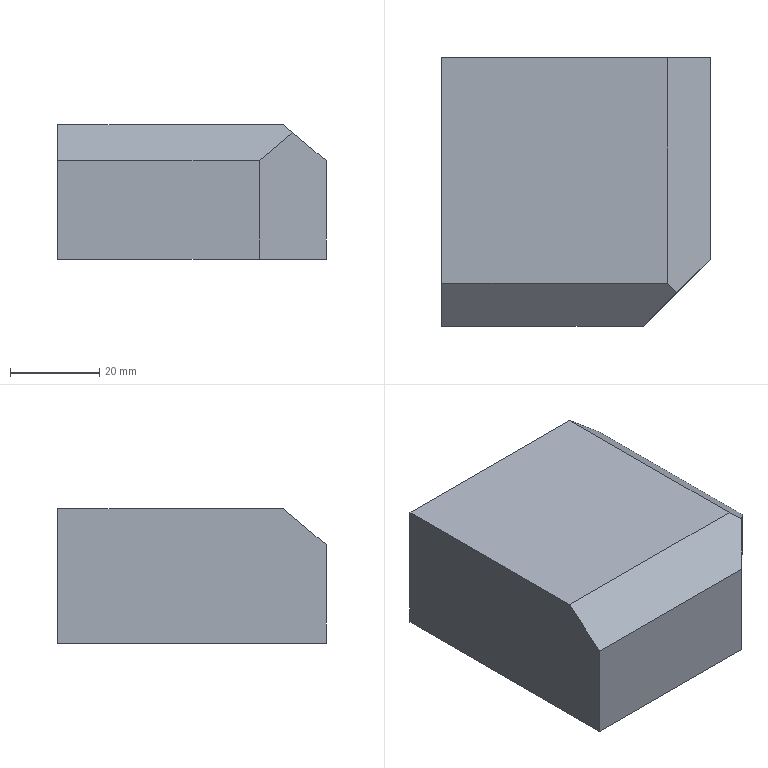Part | SolidWorks | features Chamfer 3, Extrusion 1 | 1 solid | 9 faces | box 60 x 60 x 30 mm | volume 100955 mm3 | plane 9
STEP:
#1=CARTESIAN_POINT('',(-30.,-30.,7.));
#2=VERTEX_POINT('',#1);
#3=CARTESIAN_POINT('',(-30.,-30.,-15.));
#4=VERTEX_POINT('',#3);
#5=CARTESIAN_POINT('',(-30.,-30.,15.));
#6=DIRECTION('',(0.,0.,-1.));
#7=VECTOR('',#6,1000.);
#8=LINE('',#5,#7);
#9=EDGE_CURVE('',#2,#4,#8,.T.);
#10=ORIENTED_EDGE('',*,*,#9,.F.);
#11=CARTESIAN_POINT('',(-30.,-20.466,15.));
#12=VERTEX_POINT('',#11);
#13=CARTESIAN_POINT('',(-30.,-20.466,15.));
#14=DIRECTION('',(0.,0.766,0.6428));
#15=VECTOR('',#14,1000.);
#16=LINE('',#13,#15);
#17=EDGE_CURVE('',#2,#12,#16,.T.);
#18=ORIENTED_EDGE('',*,*,#17,.T.);
#19=CARTESIAN_POINT('',(-30.,30.,15.));
#20=VERTEX_POINT('',#19);
#21=CARTESIAN_POINT('',(-30.,30.,15.));
#22=DIRECTION('',(0.,-1.,0.));
#23=VECTOR('',#22,1000.);
#24=LINE('',#21,#23);
#25=EDGE_CURVE('',#20,#12,#24,.T.);
#26=ORIENTED_EDGE('',*,*,#25,.F.);
#27=CARTESIAN_POINT('',(-30.,30.,-15.));
#28=VERTEX_POINT('',#27);
#29=CARTESIAN_POINT('',(-30.,30.,15.));
#30=DIRECTION('',(0.,0.,-1.));
#31=VECTOR('',#30,1000.);
#32=LINE('',#29,#31);
#33=EDGE_CURVE('',#20,#28,#32,.T.);
#34=ORIENTED_EDGE('',*,*,#33,.T.);
#35=CARTESIAN_POINT('',(-30.,30.,-15.));
#36=DIRECTION('',(0.,-1.,0.));
#37=VECTOR('',#36,1000.);
#38=LINE('',#35,#37);
#39=EDGE_CURVE('',#28,#4,#38,.T.);
#40=ORIENTED_EDGE('',*,*,#39,.T.);
#41=EDGE_LOOP('',(#10,#18,#26,#34,#40));
#42=FACE_OUTER_BOUND('',#41,.T.);
#43=CARTESIAN_POINT('',(-30.,30.,15.));
#44=DIRECTION('',(1.,0.,0.));
#45=DIRECTION('',(0.,1.,0.));
#46=AXIS2_PLACEMENT_3D('',#43,#44,#45);
#47=PLANE('',#46);
#48=ADVANCED_FACE('',(#42),#47,.F.);
#49=CARTESIAN_POINT('',(15.,-30.,-15.));
#50=VERTEX_POINT('',#49);
#51=CARTESIAN_POINT('',(15.,-30.,7.));
#52=VERTEX_POINT('',#51);
#53=CARTESIAN_POINT('',(15.,-30.,15.));
#54=DIRECTION('',(0.,0.,1.));
#55=VECTOR('',#54,1000.);
#56=LINE('',#53,#55);
#57=EDGE_CURVE('',#50,#52,#56,.T.);
#58=ORIENTED_EDGE('',*,*,#57,.T.);
#59=CARTESIAN_POINT('',(-30.,-30.,7.));
#60=DIRECTION('',(-1.,0.,0.));
#61=VECTOR('',#60,1000.);
#62=LINE('',#59,#61);
#63=EDGE_CURVE('',#52,#2,#62,.T.);
#64=ORIENTED_EDGE('',*,*,#63,.T.);
#65=ORIENTED_EDGE('',*,*,#9,.T.);
#66=CARTESIAN_POINT('',(-30.,-30.,-15.));
#67=DIRECTION('',(1.,0.,0.));
#68=VECTOR('',#67,1000.);
#69=LINE('',#66,#68);
#70=EDGE_CURVE('',#4,#50,#69,.T.);
#71=ORIENTED_EDGE('',*,*,#70,.T.);
#72=EDGE_LOOP('',(#58,#64,#65,#71));
#73=FACE_OUTER_BOUND('',#72,.T.);
#74=CARTESIAN_POINT('',(-30.,-30.,15.));
#75=DIRECTION('',(0.,1.,0.));
#76=DIRECTION('',(-1.,0.,0.));
#77=AXIS2_PLACEMENT_3D('',#74,#75,#76);
#78=PLANE('',#77);
#79=ADVANCED_FACE('',(#73),#78,.F.);
#80=CARTESIAN_POINT('',(30.,30.,7.));
#81=VERTEX_POINT('',#80);
#82=CARTESIAN_POINT('',(30.,30.,-15.));
#83=VERTEX_POINT('',#82);
#84=CARTESIAN_POINT('',(30.,30.,15.));
#85=DIRECTION('',(0.,0.,-1.));
#86=VECTOR('',#85,1000.);
#87=LINE('',#84,#86);
#88=EDGE_CURVE('',#81,#83,#87,.T.);
#89=ORIENTED_EDGE('',*,*,#88,.F.);
#90=CARTESIAN_POINT('',(30.,-15.,7.));
#91=VERTEX_POINT('',#90);
#92=CARTESIAN_POINT('',(30.,-15.,7.));
#93=DIRECTION('',(0.,-1.,0.));
#94=VECTOR('',#93,1000.);
#95=LINE('',#92,#94);
#96=EDGE_CURVE('',#81,#91,#95,.T.);
#97=ORIENTED_EDGE('',*,*,#96,.T.);
#98=CARTESIAN_POINT('',(30.,-15.,-15.));
#99=VERTEX_POINT('',#98);
#100=CARTESIAN_POINT('',(30.,-15.,15.));
#101=DIRECTION('',(0.,0.,-1.));
#102=VECTOR('',#101,1000.);
#103=LINE('',#100,#102);
#104=EDGE_CURVE('',#91,#99,#103,.T.);
#105=ORIENTED_EDGE('',*,*,#104,.T.);
#106=CARTESIAN_POINT('',(30.,30.,-15.));
#107=DIRECTION('',(0.,1.,0.));
#108=VECTOR('',#107,1000.);
#109=LINE('',#106,#108);
#110=EDGE_CURVE('',#99,#83,#109,.T.);
#111=ORIENTED_EDGE('',*,*,#110,.T.);
#112=EDGE_LOOP('',(#89,#97,#105,#111));
#113=FACE_OUTER_BOUND('',#112,.T.);
#114=CARTESIAN_POINT('',(30.,30.,15.));
#115=DIRECTION('',(-1.,0.,0.));
#116=DIRECTION('',(0.,-1.,0.));
#117=AXIS2_PLACEMENT_3D('',#114,#115,#116);
#118=PLANE('',#117);
#119=ADVANCED_FACE('',(#113),#118,.F.);
#120=CARTESIAN_POINT('',(20.466,30.,15.));
#121=VERTEX_POINT('',#120);
#122=CARTESIAN_POINT('',(-30.,30.,15.));
#123=DIRECTION('',(-1.,0.,0.));
#124=VECTOR('',#123,1000.);
#125=LINE('',#122,#124);
#126=EDGE_CURVE('',#121,#20,#125,.T.);
#127=ORIENTED_EDGE('',*,*,#126,.F.);
#128=CARTESIAN_POINT('',(20.466,30.,15.));
#129=DIRECTION('',(0.766,0.,-0.6428));
#130=VECTOR('',#129,1000.);
#131=LINE('',#128,#130);
#132=EDGE_CURVE('',#121,#81,#131,.T.);
#133=ORIENTED_EDGE('',*,*,#132,.T.);
#134=ORIENTED_EDGE('',*,*,#88,.T.);
#135=CARTESIAN_POINT('',(-30.,30.,-15.));
#136=DIRECTION('',(-1.,0.,0.));
#137=VECTOR('',#136,1000.);
#138=LINE('',#135,#137);
#139=EDGE_CURVE('',#83,#28,#138,.T.);
#140=ORIENTED_EDGE('',*,*,#139,.T.);
#141=ORIENTED_EDGE('',*,*,#33,.F.);
#142=EDGE_LOOP('',(#127,#133,#134,#140,#141));
#143=FACE_OUTER_BOUND('',#142,.T.);
#144=CARTESIAN_POINT('',(-30.,30.,15.));
#145=DIRECTION('',(0.,-1.,0.));
#146=DIRECTION('',(0.,0.,-1.));
#147=AXIS2_PLACEMENT_3D('',#144,#145,#146);
#148=PLANE('',#147);
#149=ADVANCED_FACE('',(#143),#148,.F.);
#150=CARTESIAN_POINT('',(20.466,-20.466,15.));
#151=VERTEX_POINT('',#150);
#152=CARTESIAN_POINT('',(15.,-20.466,15.));
#153=DIRECTION('',(1.,0.,0.));
#154=VECTOR('',#153,1000.);
#155=LINE('',#152,#154);
#156=EDGE_CURVE('',#12,#151,#155,.T.);
#157=ORIENTED_EDGE('',*,*,#156,.T.);
#158=CARTESIAN_POINT('',(20.466,30.,15.));
#159=DIRECTION('',(0.,1.,0.));
#160=VECTOR('',#159,1000.);
#161=LINE('',#158,#160);
#162=EDGE_CURVE('',#151,#121,#161,.T.);
#163=ORIENTED_EDGE('',*,*,#162,.T.);
#164=ORIENTED_EDGE('',*,*,#126,.T.);
#165=ORIENTED_EDGE('',*,*,#25,.T.);
#166=EDGE_LOOP('',(#157,#163,#164,#165));
#167=FACE_OUTER_BOUND('',#166,.T.);
#168=CARTESIAN_POINT('',(-30.,-30.,15.));
#169=DIRECTION('',(0.,0.,1.));
#170=DIRECTION('',(1.,0.,0.));
#171=AXIS2_PLACEMENT_3D('',#168,#169,#170);
#172=PLANE('',#171);
#173=ADVANCED_FACE('',(#167),#172,.T.);
#174=ORIENTED_EDGE('',*,*,#110,.F.);
#175=CARTESIAN_POINT('',(30.,-15.,-15.));
#176=DIRECTION('',(-0.7071,-0.7071,0.));
#177=VECTOR('',#176,1000.);
#178=LINE('',#175,#177);
#179=EDGE_CURVE('',#99,#50,#178,.T.);
#180=ORIENTED_EDGE('',*,*,#179,.T.);
#181=ORIENTED_EDGE('',*,*,#70,.F.);
#182=ORIENTED_EDGE('',*,*,#39,.F.);
#183=ORIENTED_EDGE('',*,*,#139,.F.);
#184=EDGE_LOOP('',(#174,#180,#181,#182,#183));
#185=FACE_OUTER_BOUND('',#184,.T.);
#186=CARTESIAN_POINT('',(-30.,-30.,-15.));
#187=DIRECTION('',(0.,0.,1.));
#188=DIRECTION('',(1.,0.,0.));
#189=AXIS2_PLACEMENT_3D('',#186,#187,#188);
#190=PLANE('',#189);
#191=ADVANCED_FACE('',(#185),#190,.F.);
#192=ORIENTED_EDGE('',*,*,#104,.F.);
#193=CARTESIAN_POINT('',(22.5,-22.5,13.293));
#194=VERTEX_POINT('',#193);
#195=CARTESIAN_POINT('',(27.518,-17.482,9.083));
#196=DIRECTION('',(-0.6081,-0.6081,0.5103));
#197=VECTOR('',#196,1000.);
#198=LINE('',#195,#197);
#199=EDGE_CURVE('',#91,#194,#198,.T.);
#200=ORIENTED_EDGE('',*,*,#199,.T.);
#201=CARTESIAN_POINT('',(28.577,-16.423,18.392));
#202=DIRECTION('',(-0.6081,-0.6081,-0.5103));
#203=VECTOR('',#202,1000.);
#204=LINE('',#201,#203);
#205=EDGE_CURVE('',#194,#52,#204,.T.);
#206=ORIENTED_EDGE('',*,*,#205,.T.);
#207=ORIENTED_EDGE('',*,*,#57,.F.);
#208=ORIENTED_EDGE('',*,*,#179,.F.);
#209=EDGE_LOOP('',(#192,#200,#206,#207,#208));
#210=FACE_OUTER_BOUND('',#209,.T.);
#211=CARTESIAN_POINT('',(30.,-15.,15.));
#212=DIRECTION('',(-0.7071,0.7071,0.));
#213=DIRECTION('',(-0.7071,-0.7071,0.));
#214=AXIS2_PLACEMENT_3D('',#211,#212,#213);
#215=PLANE('',#214);
#216=ADVANCED_FACE('',(#210),#215,.F.);
#217=ORIENTED_EDGE('',*,*,#205,.F.);
#218=CARTESIAN_POINT('',(1.803,-1.803,30.66));
#219=DIRECTION('',(-0.6081,0.6081,0.5103));
#220=VECTOR('',#219,1000.);
#221=LINE('',#218,#220);
#222=EDGE_CURVE('',#194,#151,#221,.T.);
#223=ORIENTED_EDGE('',*,*,#222,.T.);
#224=ORIENTED_EDGE('',*,*,#156,.F.);
#225=ORIENTED_EDGE('',*,*,#17,.F.);
#226=ORIENTED_EDGE('',*,*,#63,.F.);
#227=EDGE_LOOP('',(#217,#223,#224,#225,#226));
#228=FACE_OUTER_BOUND('',#227,.T.);
#229=CARTESIAN_POINT('',(-30.,-20.466,15.));
#230=DIRECTION('',(0.,-0.6428,0.766));
#231=DIRECTION('',(0.,-0.766,-0.6428));
#232=AXIS2_PLACEMENT_3D('',#229,#230,#231);
#233=PLANE('',#232);
#234=ADVANCED_FACE('',(#228),#233,.T.);
#235=ORIENTED_EDGE('',*,*,#199,.F.);
#236=ORIENTED_EDGE('',*,*,#96,.F.);
#237=ORIENTED_EDGE('',*,*,#132,.F.);
#238=ORIENTED_EDGE('',*,*,#162,.F.);
#239=ORIENTED_EDGE('',*,*,#222,.F.);
#240=EDGE_LOOP('',(#235,#236,#237,#238,#239));
#241=FACE_OUTER_BOUND('',#240,.T.);
#242=CARTESIAN_POINT('',(20.466,-30.,15.));
#243=DIRECTION('',(0.6428,0.,0.766));
#244=DIRECTION('',(0.766,0.,-0.6428));
#245=AXIS2_PLACEMENT_3D('',#242,#243,#244);
#246=PLANE('',#245);
#247=ADVANCED_FACE('',(#241),#246,.T.);
#248=CLOSED_SHELL('',(#48,#79,#119,#149,#173,#191,#216,#234,#247));
#249=MANIFOLD_SOLID_BREP('',#248);
#250=CARTESIAN_POINT('',(0.,0.,0.));
#251=DIRECTION('',(0.,0.,1.));
#252=DIRECTION('',(1.,0.,0.));
#253=AXIS2_PLACEMENT_3D('',#250,#251,#252);
#254=(LENGTH_UNIT()NAMED_UNIT(*)SI_UNIT(.MILLI.,.METRE.));
#255=UNCERTAINTY_MEASURE_WITH_UNIT(LENGTH_MEASURE(0.00001),#254,'','');
#256=(NAMED_UNIT(*)PLANE_ANGLE_UNIT()SI_UNIT($,.RADIAN.));
#257=(NAMED_UNIT(*)SI_UNIT($,.STERADIAN.)SOLID_ANGLE_UNIT());
#258=(GEOMETRIC_REPRESENTATION_CONTEXT(3)GLOBAL_UNCERTAINTY_ASSIGNED_CONTEXT((#255))GLOBAL_UNIT_ASSIGNED_CONTEXT((#254,#256,#257))REPRESENTATION_CONTEXT('',''));
#259=ADVANCED_BREP_SHAPE_REPRESENTATION('',(#249,#253),#258);